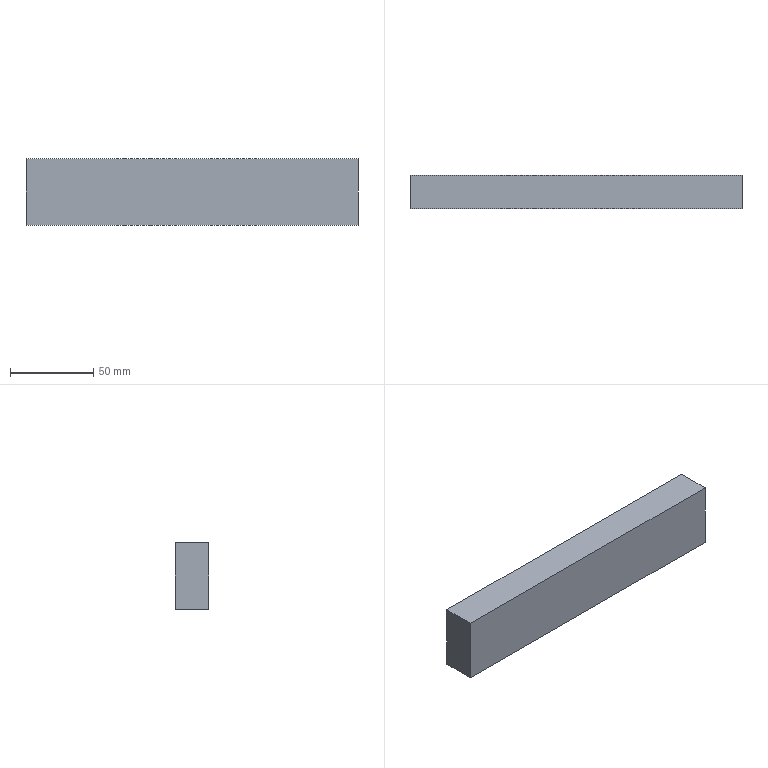Part | SolidWorks | features Extrusion 1 | 1 solid | 6 faces | box 199 x 20 x 40 mm | volume 159200 mm3 | plane 6
STEP:
#1=CARTESIAN_POINT('',(0.,0.,-40.));
#2=VERTEX_POINT('',#1);
#3=CARTESIAN_POINT('',(0.,0.,0.));
#4=VERTEX_POINT('',#3);
#5=CARTESIAN_POINT('',(0.,0.,0.));
#6=DIRECTION('',(0.,0.,1.));
#7=VECTOR('',#6,1000.);
#8=LINE('',#5,#7);
#9=EDGE_CURVE('',#2,#4,#8,.T.);
#10=ORIENTED_EDGE('',*,*,#9,.T.);
#11=CARTESIAN_POINT('',(0.,20.,0.));
#12=VERTEX_POINT('',#11);
#13=CARTESIAN_POINT('',(0.,20.,0.));
#14=DIRECTION('',(0.,-1.,0.));
#15=VECTOR('',#14,1000.);
#16=LINE('',#13,#15);
#17=EDGE_CURVE('',#12,#4,#16,.T.);
#18=ORIENTED_EDGE('',*,*,#17,.F.);
#19=CARTESIAN_POINT('',(0.,20.,-40.));
#20=VERTEX_POINT('',#19);
#21=CARTESIAN_POINT('',(0.,20.,0.));
#22=DIRECTION('',(0.,0.,1.));
#23=VECTOR('',#22,1000.);
#24=LINE('',#21,#23);
#25=EDGE_CURVE('',#20,#12,#24,.T.);
#26=ORIENTED_EDGE('',*,*,#25,.F.);
#27=CARTESIAN_POINT('',(0.,20.,-40.));
#28=DIRECTION('',(0.,-1.,0.));
#29=VECTOR('',#28,1000.);
#30=LINE('',#27,#29);
#31=EDGE_CURVE('',#20,#2,#30,.T.);
#32=ORIENTED_EDGE('',*,*,#31,.T.);
#33=EDGE_LOOP('',(#10,#18,#26,#32));
#34=FACE_OUTER_BOUND('',#33,.T.);
#35=CARTESIAN_POINT('',(0.,20.,0.));
#36=DIRECTION('',(1.,0.,0.));
#37=DIRECTION('',(0.,0.,-1.));
#38=AXIS2_PLACEMENT_3D('',#35,#36,#37);
#39=PLANE('',#38);
#40=ADVANCED_FACE('',(#34),#39,.F.);
#41=CARTESIAN_POINT('',(199.,0.,0.));
#42=VERTEX_POINT('',#41);
#43=CARTESIAN_POINT('',(0.,0.,0.));
#44=DIRECTION('',(1.,0.,0.));
#45=VECTOR('',#44,1000.);
#46=LINE('',#43,#45);
#47=EDGE_CURVE('',#4,#42,#46,.T.);
#48=ORIENTED_EDGE('',*,*,#47,.T.);
#49=CARTESIAN_POINT('',(199.,20.,0.));
#50=VERTEX_POINT('',#49);
#51=CARTESIAN_POINT('',(199.,20.,0.));
#52=DIRECTION('',(0.,-1.,0.));
#53=VECTOR('',#52,1000.);
#54=LINE('',#51,#53);
#55=EDGE_CURVE('',#50,#42,#54,.T.);
#56=ORIENTED_EDGE('',*,*,#55,.F.);
#57=CARTESIAN_POINT('',(0.,20.,0.));
#58=DIRECTION('',(1.,0.,0.));
#59=VECTOR('',#58,1000.);
#60=LINE('',#57,#59);
#61=EDGE_CURVE('',#12,#50,#60,.T.);
#62=ORIENTED_EDGE('',*,*,#61,.F.);
#63=ORIENTED_EDGE('',*,*,#17,.T.);
#64=EDGE_LOOP('',(#48,#56,#62,#63));
#65=FACE_OUTER_BOUND('',#64,.T.);
#66=CARTESIAN_POINT('',(0.,20.,0.));
#67=DIRECTION('',(0.,0.,-1.));
#68=DIRECTION('',(-1.,0.,0.));
#69=AXIS2_PLACEMENT_3D('',#66,#67,#68);
#70=PLANE('',#69);
#71=ADVANCED_FACE('',(#65),#70,.F.);
#72=CARTESIAN_POINT('',(199.,0.,-40.));
#73=VERTEX_POINT('',#72);
#74=CARTESIAN_POINT('',(199.,0.,0.));
#75=DIRECTION('',(0.,0.,-1.));
#76=VECTOR('',#75,1000.);
#77=LINE('',#74,#76);
#78=EDGE_CURVE('',#42,#73,#77,.T.);
#79=ORIENTED_EDGE('',*,*,#78,.T.);
#80=CARTESIAN_POINT('',(199.,20.,-40.));
#81=VERTEX_POINT('',#80);
#82=CARTESIAN_POINT('',(199.,20.,-40.));
#83=DIRECTION('',(0.,-1.,0.));
#84=VECTOR('',#83,1000.);
#85=LINE('',#82,#84);
#86=EDGE_CURVE('',#81,#73,#85,.T.);
#87=ORIENTED_EDGE('',*,*,#86,.F.);
#88=CARTESIAN_POINT('',(199.,20.,0.));
#89=DIRECTION('',(0.,0.,-1.));
#90=VECTOR('',#89,1000.);
#91=LINE('',#88,#90);
#92=EDGE_CURVE('',#50,#81,#91,.T.);
#93=ORIENTED_EDGE('',*,*,#92,.F.);
#94=ORIENTED_EDGE('',*,*,#55,.T.);
#95=EDGE_LOOP('',(#79,#87,#93,#94));
#96=FACE_OUTER_BOUND('',#95,.T.);
#97=CARTESIAN_POINT('',(199.,20.,0.));
#98=DIRECTION('',(-1.,0.,0.));
#99=DIRECTION('',(0.,0.,1.));
#100=AXIS2_PLACEMENT_3D('',#97,#98,#99);
#101=PLANE('',#100);
#102=ADVANCED_FACE('',(#96),#101,.F.);
#103=CARTESIAN_POINT('',(0.,0.,-40.));
#104=DIRECTION('',(-1.,0.,0.));
#105=VECTOR('',#104,1000.);
#106=LINE('',#103,#105);
#107=EDGE_CURVE('',#73,#2,#106,.T.);
#108=ORIENTED_EDGE('',*,*,#107,.T.);
#109=ORIENTED_EDGE('',*,*,#31,.F.);
#110=CARTESIAN_POINT('',(0.,20.,-40.));
#111=DIRECTION('',(-1.,0.,0.));
#112=VECTOR('',#111,1000.);
#113=LINE('',#110,#112);
#114=EDGE_CURVE('',#81,#20,#113,.T.);
#115=ORIENTED_EDGE('',*,*,#114,.F.);
#116=ORIENTED_EDGE('',*,*,#86,.T.);
#117=EDGE_LOOP('',(#108,#109,#115,#116));
#118=FACE_OUTER_BOUND('',#117,.T.);
#119=CARTESIAN_POINT('',(0.,20.,-40.));
#120=DIRECTION('',(0.,0.,1.));
#121=DIRECTION('',(1.,0.,0.));
#122=AXIS2_PLACEMENT_3D('',#119,#120,#121);
#123=PLANE('',#122);
#124=ADVANCED_FACE('',(#118),#123,.F.);
#125=ORIENTED_EDGE('',*,*,#25,.T.);
#126=ORIENTED_EDGE('',*,*,#61,.T.);
#127=ORIENTED_EDGE('',*,*,#92,.T.);
#128=ORIENTED_EDGE('',*,*,#114,.T.);
#129=EDGE_LOOP('',(#125,#126,#127,#128));
#130=FACE_OUTER_BOUND('',#129,.T.);
#131=CARTESIAN_POINT('',(0.,20.,-40.));
#132=DIRECTION('',(0.,-1.,0.));
#133=DIRECTION('',(0.,0.,-1.));
#134=AXIS2_PLACEMENT_3D('',#131,#132,#133);
#135=PLANE('',#134);
#136=ADVANCED_FACE('',(#130),#135,.F.);
#137=ORIENTED_EDGE('',*,*,#9,.F.);
#138=ORIENTED_EDGE('',*,*,#107,.F.);
#139=ORIENTED_EDGE('',*,*,#78,.F.);
#140=ORIENTED_EDGE('',*,*,#47,.F.);
#141=EDGE_LOOP('',(#137,#138,#139,#140));
#142=FACE_OUTER_BOUND('',#141,.T.);
#143=CARTESIAN_POINT('',(0.,0.,-40.));
#144=DIRECTION('',(0.,-1.,0.));
#145=DIRECTION('',(0.,0.,-1.));
#146=AXIS2_PLACEMENT_3D('',#143,#144,#145);
#147=PLANE('',#146);
#148=ADVANCED_FACE('',(#142),#147,.T.);
#149=CLOSED_SHELL('',(#40,#71,#102,#124,#136,#148));
#150=MANIFOLD_SOLID_BREP('',#149);
#151=CARTESIAN_POINT('',(0.,0.,0.));
#152=DIRECTION('',(0.,0.,1.));
#153=DIRECTION('',(1.,0.,0.));
#154=AXIS2_PLACEMENT_3D('',#151,#152,#153);
#155=(LENGTH_UNIT()NAMED_UNIT(*)SI_UNIT(.MILLI.,.METRE.));
#156=UNCERTAINTY_MEASURE_WITH_UNIT(LENGTH_MEASURE(0.00001),#155,'','');
#157=(NAMED_UNIT(*)PLANE_ANGLE_UNIT()SI_UNIT($,.RADIAN.));
#158=(NAMED_UNIT(*)SI_UNIT($,.STERADIAN.)SOLID_ANGLE_UNIT());
#159=(GEOMETRIC_REPRESENTATION_CONTEXT(3)GLOBAL_UNCERTAINTY_ASSIGNED_CONTEXT((#156))GLOBAL_UNIT_ASSIGNED_CONTEXT((#155,#157,#158))REPRESENTATION_CONTEXT('',''));
#160=ADVANCED_BREP_SHAPE_REPRESENTATION('',(#150,#154),#159);